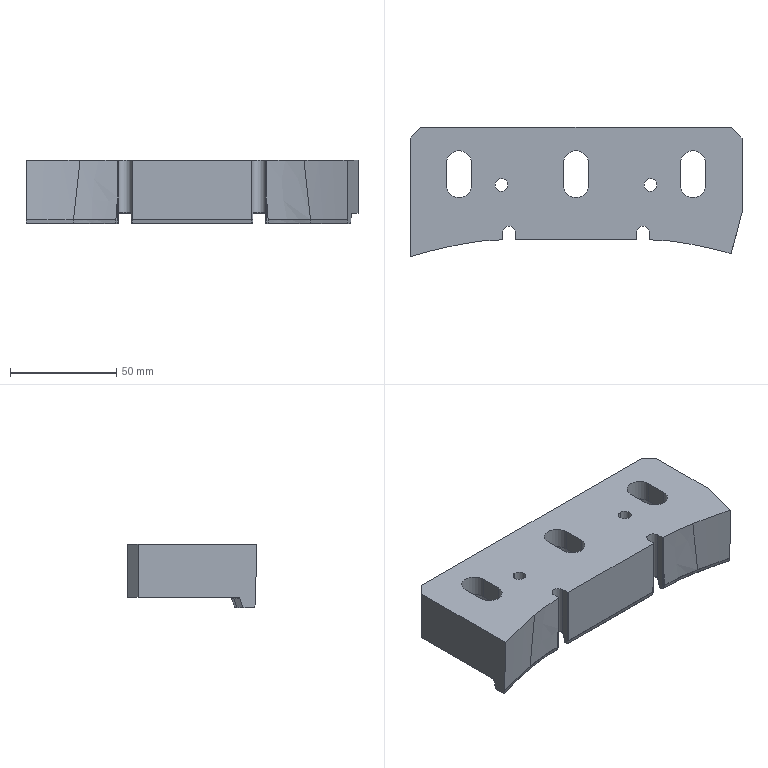NC program | Mastercam | posted with a generic post | part box 156 x 60.706 x 30 mm
Lines 11307 to 11458 of 78092:
N4120 T11 M6
N4130 G0 G90 G17 G54 X-91. Y-5.5 A0. S1800 M3
N4140 G43 H11 Z50.
N4150 Z10.3
N4160 G1 Z-14.85 F600.
N4170 X-86. F500.
N4180 G3 X-83. Y-2.5 I0. J3.
N4190 G1 Y25.353
N4200 G2 X-81.536 Y28.888 I5. J0.
N4210 G1 X-76.536 Y33.888
N4220 G2 X-73. Y35.353 I3.536 J-3.535
N4230 G1 X73.
N4240 G2 X76.536 Y33.888 I0. J-5.
N4250 G1 X81.536 Y28.888
N4260 G2 X83. Y25.353 I-3.536 J-3.535
N4270 G1 Y-10.439
N4280 X77.701 Y-30.214
N4290 G2 X72.872 Y-33.919 I-4.829 J1.294
N4300 X71.572 Y-33.748 I0. J4.999
N4310 G3 X51.693 Y-29.18 I-71.572 J-265.899
N4320 G1 X47.439 Y-28.465
N4330 X43.32 Y-27.959
N4340 X39.134 Y-27.629
N4350 X34.753 Y-27.477
N4360 X34.393 Y-27.455
N4370 X33.861 Y-27.37
N4380 X33.342 Y-27.233
N4390 X32.84 Y-27.047
N4400 X32.359 Y-26.814
N4410 X31.901 Y-26.534
N4420 X31.494 Y-26.227
N4430 X30.78 Y-26.951
N4440 X28.59 Y-27.475
N4450 X-28.574
N4460 X-30.729 Y-26.973
N4470 X-31.489 Y-26.223
N4480 X-31.908 Y-26.538
N4490 X-32.364 Y-26.817
N4500 X-32.846 Y-27.05
N4510 X-33.349 Y-27.235
N4520 X-33.986 Y-27.402
N4530 X-34.632 Y-27.473
N4540 X-39.188 Y-27.632
N4550 X-43.319 Y-27.959
N4560 X-47.488 Y-28.473
N4570 X-51.693 Y-29.18
N4580 G3 X-76.609 Y-35.156 I51.693 J-270.467
N4590 G2 X-78. Y-35.353 I-1.391 J4.803
N4600 X-83. Y-30.353 I0. J5.
N4610 G1 Y-2.5
N4620 G3 X-86. Y.5 I-3. J0.
N4630 G1 X-91.
N4640 G0 Z25.
N4650 Y-5.5
N4660 Z-4.85
N4670 G1 Z-30. F600.
N4680 X-86. F500.
N4690 G3 X-83. Y-2.5 I0. J3.
N4700 G1 Y25.353
N4710 G2 X-81.536 Y28.888 I5. J0.
N4720 G1 X-76.536 Y33.888
N4730 G2 X-73. Y35.353 I3.536 J-3.535
N4740 G1 X73.
N4750 G2 X76.536 Y33.888 I0. J-5.
N4760 G1 X81.536 Y28.888
N4770 G2 X83. Y25.353 I-3.536 J-3.535
N4780 G1 Y-10.439
N4790 X77.701 Y-30.214
N4800 G2 X72.872 Y-33.919 I-4.829 J1.294
N4810 X71.572 Y-33.748 I0. J4.999
N4820 G3 X51.693 Y-29.18 I-71.572 J-265.899
N4830 G1 X47.439 Y-28.465
N4840 X43.32 Y-27.959
N4850 X39.134 Y-27.629
N4860 X34.753 Y-27.477
N4870 X34.393 Y-27.455
N4880 X33.861 Y-27.37
N4890 X33.342 Y-27.233
N4900 X32.84 Y-27.047
N4910 X32.359 Y-26.814
N4920 X31.901 Y-26.534
N4930 X31.494 Y-26.227
N4940 X30.78 Y-26.951
N4950 X28.59 Y-27.475
N4960 X-28.574
N4970 X-30.729 Y-26.973
N4980 X-31.489 Y-26.223
N4990 X-31.908 Y-26.538
N5000 X-32.364 Y-26.817
N5010 X-32.846 Y-27.05
N5020 X-33.349 Y-27.235
N5030 X-33.986 Y-27.402
N5040 X-34.632 Y-27.473
N5050 X-39.188 Y-27.632
N5060 X-43.319 Y-27.959
N5070 X-47.488 Y-28.473
N5080 X-51.693 Y-29.18
N5090 G3 X-76.609 Y-35.156 I51.693 J-270.467
N5100 G2 X-78. Y-35.353 I-1.391 J4.803
N5110 X-83. Y-30.353 I0. J5.
N5120 G1 Y-2.5
N5130 G3 X-86. Y.5 I-3. J0.
N5140 G1 X-91.
N5150 G0 Z50.
N5160 S1600 M3
N5170 M8
N5180 X-54.7 Y13.553
N5190 Z10.3
N5200 G1 Z-15. F600.
N5210 Y14.053 F400.
N5220 G3 X-55. Y14.353 I-.3 J0.
N5230 X-56. Y13.353 I0. J-1.
N5240 G1 Y3.353
N5250 G3 X-55. Y2.353 I1. J0.
N5260 X-54. Y3.353 I0. J1.
N5270 G1 Y13.353
N5280 G3 X-55. Y14.353 I-1. J0.
N5290 X-55.3 Y14.053 I0. J-.3
N5300 G1 Y13.553
N5310 G0 Z50.
N5320 X.3
N5330 Z10.3
N5340 G1 Z-15. F600.
N5350 Y14.053 F400.
N5360 G3 X0. Y14.353 I-.3 J0.
N5370 X-1. Y13.353 I0. J-1.
N5380 G1 Y3.353
N5390 G3 X0. Y2.353 I1. J0.
N5400 X1. Y3.353 I0. J1.
N5410 G1 Y13.353
N5420 G3 X0. Y14.353 I-1. J0.
N5430 X-.3 Y14.053 I0. J-.3
N5440 G1 Y13.553
N5450 G0 Z50.
N5460 X55.3
N5470 Z10.3
N5480 G1 Z-15. F600.
N5490 Y14.053 F400.
N5500 G3 X55. Y14.353 I-.3 J0.
N5510 X54. Y13.353 I0. J-1.
N5520 G1 Y3.353
N5530 G3 X55. Y2.353 I1. J0.
N5540 X56. Y3.353 I0. J1.
N5550 G1 Y13.353
N5560 G3 X55. Y14.353 I-1. J0.
N5570 X54.7 Y14.053 I0. J-.3
N5580 G1 Y13.553
N5590 G0 Z50.
N5600 M5
N5610 G91 G28 Z0. M9
N5620 A0.
N5630 M01